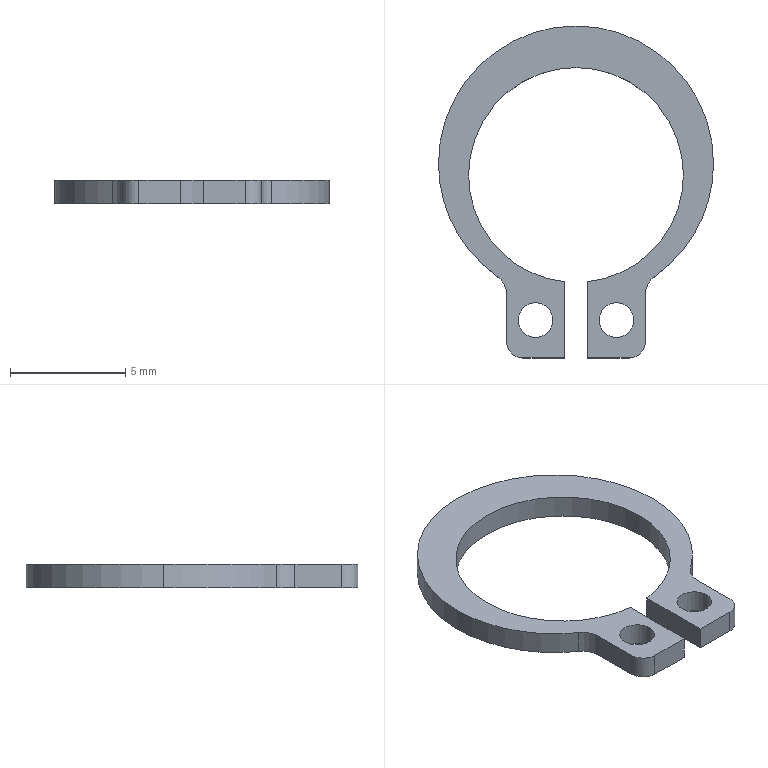Part | SolidWorks | features MoveCopyBody 1, Stock 1 | 1 solid | 22 faces | box 11.91 x 14.373 x 1 mm | volume 52.893 mm3 | cylinder 14 | plane 8 | commonest cylinder face diameters 1.5 x4 9.3 x3 11.91 x3 1.4 x2 2 x2
STEP:
#1=CARTESIAN_POINT('',(1.,-6.286,1.));
#2=VERTEX_POINT('',#1);
#3=CARTESIAN_POINT('',(2.5,-6.286,1.));
#4=VERTEX_POINT('',#3);
#5=CARTESIAN_POINT('',(1.75,-6.286,1.));
#6=DIRECTION('',(0.,0.,1.));
#7=DIRECTION('',(-1.,0.,0.));
#8=AXIS2_PLACEMENT_3D('',#5,#6,#7);
#9=CIRCLE('',#8,0.75);
#10=EDGE_CURVE('',#2,#4,#9,.T.);
#11=ORIENTED_EDGE('',*,*,#10,.T.);
#12=CARTESIAN_POINT('',(2.5,-6.286,0.));
#13=VERTEX_POINT('',#12);
#14=CARTESIAN_POINT('',(2.5,-6.286,1.));
#15=DIRECTION('',(0.,0.,-1.));
#16=VECTOR('',#15,1000.);
#17=LINE('',#14,#16);
#18=EDGE_CURVE('',#4,#13,#17,.T.);
#19=ORIENTED_EDGE('',*,*,#18,.T.);
#20=CARTESIAN_POINT('',(1.,-6.286,0.));
#21=VERTEX_POINT('',#20);
#22=CARTESIAN_POINT('',(1.75,-6.286,0.));
#23=DIRECTION('',(0.,0.,1.));
#24=DIRECTION('',(-1.,0.,0.));
#25=AXIS2_PLACEMENT_3D('',#22,#23,#24);
#26=CIRCLE('',#25,0.75);
#27=EDGE_CURVE('',#21,#13,#26,.T.);
#28=ORIENTED_EDGE('',*,*,#27,.F.);
#29=CARTESIAN_POINT('',(1.,-6.286,1.));
#30=DIRECTION('',(0.,0.,-1.));
#31=VECTOR('',#30,1000.);
#32=LINE('',#29,#31);
#33=EDGE_CURVE('',#2,#21,#32,.T.);
#34=ORIENTED_EDGE('',*,*,#33,.F.);
#35=EDGE_LOOP('',(#11,#19,#28,#34));
#36=FACE_OUTER_BOUND('',#35,.T.);
#37=CARTESIAN_POINT('',(1.75,-6.286,1.));
#38=DIRECTION('',(0.,0.,-1.));
#39=DIRECTION('',(-1.,0.,0.));
#40=AXIS2_PLACEMENT_3D('',#37,#38,#39);
#41=CYLINDRICAL_SURFACE('',#40,0.75);
#42=ADVANCED_FACE('',(#36),#41,.F.);
#43=CARTESIAN_POINT('',(-2.5,-6.286,1.));
#44=VERTEX_POINT('',#43);
#45=CARTESIAN_POINT('',(-1.,-6.286,1.));
#46=VERTEX_POINT('',#45);
#47=CARTESIAN_POINT('',(-1.75,-6.286,1.));
#48=DIRECTION('',(0.,0.,1.));
#49=DIRECTION('',(1.,0.,0.));
#50=AXIS2_PLACEMENT_3D('',#47,#48,#49);
#51=CIRCLE('',#50,0.75);
#52=EDGE_CURVE('',#44,#46,#51,.T.);
#53=ORIENTED_EDGE('',*,*,#52,.T.);
#54=CARTESIAN_POINT('',(-1.,-6.286,0.));
#55=VERTEX_POINT('',#54);
#56=CARTESIAN_POINT('',(-1.,-6.286,1.));
#57=DIRECTION('',(0.,0.,-1.));
#58=VECTOR('',#57,1000.);
#59=LINE('',#56,#58);
#60=EDGE_CURVE('',#46,#55,#59,.T.);
#61=ORIENTED_EDGE('',*,*,#60,.T.);
#62=CARTESIAN_POINT('',(-2.5,-6.286,0.));
#63=VERTEX_POINT('',#62);
#64=CARTESIAN_POINT('',(-1.75,-6.286,0.));
#65=DIRECTION('',(0.,0.,1.));
#66=DIRECTION('',(1.,0.,0.));
#67=AXIS2_PLACEMENT_3D('',#64,#65,#66);
#68=CIRCLE('',#67,0.75);
#69=EDGE_CURVE('',#63,#55,#68,.T.);
#70=ORIENTED_EDGE('',*,*,#69,.F.);
#71=CARTESIAN_POINT('',(-2.5,-6.286,1.));
#72=DIRECTION('',(0.,0.,-1.));
#73=VECTOR('',#72,1000.);
#74=LINE('',#71,#73);
#75=EDGE_CURVE('',#44,#63,#74,.T.);
#76=ORIENTED_EDGE('',*,*,#75,.F.);
#77=EDGE_LOOP('',(#53,#61,#70,#76));
#78=FACE_OUTER_BOUND('',#77,.T.);
#79=CARTESIAN_POINT('',(-1.75,-6.286,1.));
#80=DIRECTION('',(0.,0.,-1.));
#81=DIRECTION('',(-1.,0.,0.));
#82=AXIS2_PLACEMENT_3D('',#79,#80,#81);
#83=CYLINDRICAL_SURFACE('',#82,0.75);
#84=ADVANCED_FACE('',(#78),#83,.F.);
#85=CARTESIAN_POINT('',(5.955,0.495,1.));
#86=VERTEX_POINT('',#85);
#87=CARTESIAN_POINT('',(-5.955,0.495,1.));
#88=VERTEX_POINT('',#87);
#89=CARTESIAN_POINT('',(0.,0.495,1.));
#90=DIRECTION('',(0.,0.,1.));
#91=DIRECTION('',(1.,0.,0.));
#92=AXIS2_PLACEMENT_3D('',#89,#90,#91);
#93=CIRCLE('',#92,5.955);
#94=EDGE_CURVE('',#86,#88,#93,.T.);
#95=ORIENTED_EDGE('',*,*,#94,.F.);
#96=CARTESIAN_POINT('',(5.955,0.495,0.));
#97=VERTEX_POINT('',#96);
#98=CARTESIAN_POINT('',(5.955,0.495,1.));
#99=DIRECTION('',(0.,0.,-1.));
#100=VECTOR('',#99,1000.);
#101=LINE('',#98,#100);
#102=EDGE_CURVE('',#86,#97,#101,.T.);
#103=ORIENTED_EDGE('',*,*,#102,.T.);
#104=CARTESIAN_POINT('',(-5.955,0.495,0.));
#105=VERTEX_POINT('',#104);
#106=CARTESIAN_POINT('',(0.,0.495,0.));
#107=DIRECTION('',(0.,0.,1.));
#108=DIRECTION('',(1.,0.,0.));
#109=AXIS2_PLACEMENT_3D('',#106,#107,#108);
#110=CIRCLE('',#109,5.955);
#111=EDGE_CURVE('',#97,#105,#110,.T.);
#112=ORIENTED_EDGE('',*,*,#111,.T.);
#113=CARTESIAN_POINT('',(-5.955,0.495,1.));
#114=DIRECTION('',(0.,0.,-1.));
#115=VECTOR('',#114,1000.);
#116=LINE('',#113,#115);
#117=EDGE_CURVE('',#88,#105,#116,.T.);
#118=ORIENTED_EDGE('',*,*,#117,.F.);
#119=EDGE_LOOP('',(#95,#103,#112,#118));
#120=FACE_OUTER_BOUND('',#119,.T.);
#121=CARTESIAN_POINT('',(0.,0.495,1.));
#122=DIRECTION('',(0.,0.,-1.));
#123=DIRECTION('',(-1.,0.,0.));
#124=AXIS2_PLACEMENT_3D('',#121,#122,#123);
#125=CYLINDRICAL_SURFACE('',#124,5.955);
#126=ADVANCED_FACE('',(#120),#125,.T.);
#127=CARTESIAN_POINT('',(-3.425,-4.377,1.));
#128=VERTEX_POINT('',#127);
#129=CARTESIAN_POINT('',(0.,0.495,1.));
#130=DIRECTION('',(0.,0.,1.));
#131=DIRECTION('',(1.,0.,0.));
#132=AXIS2_PLACEMENT_3D('',#129,#130,#131);
#133=CIRCLE('',#132,5.955);
#134=EDGE_CURVE('',#88,#128,#133,.T.);
#135=ORIENTED_EDGE('',*,*,#134,.F.);
#136=ORIENTED_EDGE('',*,*,#117,.T.);
#137=CARTESIAN_POINT('',(-3.425,-4.377,0.));
#138=VERTEX_POINT('',#137);
#139=CARTESIAN_POINT('',(0.,0.495,0.));
#140=DIRECTION('',(0.,0.,1.));
#141=DIRECTION('',(1.,0.,0.));
#142=AXIS2_PLACEMENT_3D('',#139,#140,#141);
#143=CIRCLE('',#142,5.955);
#144=EDGE_CURVE('',#105,#138,#143,.T.);
#145=ORIENTED_EDGE('',*,*,#144,.T.);
#146=CARTESIAN_POINT('',(-3.425,-4.377,1.));
#147=DIRECTION('',(0.,0.,1.));
#148=VECTOR('',#147,1000.);
#149=LINE('',#146,#148);
#150=EDGE_CURVE('',#138,#128,#149,.T.);
#151=ORIENTED_EDGE('',*,*,#150,.T.);
#152=EDGE_LOOP('',(#135,#136,#145,#151));
#153=FACE_OUTER_BOUND('',#152,.T.);
#154=CARTESIAN_POINT('',(0.,0.495,1.));
#155=DIRECTION('',(0.,0.,-1.));
#156=DIRECTION('',(-1.,0.,0.));
#157=AXIS2_PLACEMENT_3D('',#154,#155,#156);
#158=CYLINDRICAL_SURFACE('',#157,5.955);
#159=ADVANCED_FACE('',(#153),#158,.T.);
#160=CARTESIAN_POINT('',(4.65,0.,1.));
#161=VERTEX_POINT('',#160);
#162=CARTESIAN_POINT('',(0.5,-4.623,1.));
#163=VERTEX_POINT('',#162);
#164=CARTESIAN_POINT('',(0.,0.,1.));
#165=DIRECTION('',(0.,0.,-1.));
#166=DIRECTION('',(1.,0.,0.));
#167=AXIS2_PLACEMENT_3D('',#164,#165,#166);
#168=CIRCLE('',#167,4.65);
#169=EDGE_CURVE('',#161,#163,#168,.T.);
#170=ORIENTED_EDGE('',*,*,#169,.F.);
#171=CARTESIAN_POINT('',(4.65,0.,0.));
#172=VERTEX_POINT('',#171);
#173=CARTESIAN_POINT('',(4.65,0.,1.));
#174=DIRECTION('',(0.,0.,-1.));
#175=VECTOR('',#174,1000.);
#176=LINE('',#173,#175);
#177=EDGE_CURVE('',#161,#172,#176,.T.);
#178=ORIENTED_EDGE('',*,*,#177,.T.);
#179=CARTESIAN_POINT('',(0.5,-4.623,0.));
#180=VERTEX_POINT('',#179);
#181=CARTESIAN_POINT('',(0.,0.,0.));
#182=DIRECTION('',(0.,0.,-1.));
#183=DIRECTION('',(1.,0.,0.));
#184=AXIS2_PLACEMENT_3D('',#181,#182,#183);
#185=CIRCLE('',#184,4.65);
#186=EDGE_CURVE('',#172,#180,#185,.T.);
#187=ORIENTED_EDGE('',*,*,#186,.T.);
#188=CARTESIAN_POINT('',(0.5,-4.623,1.));
#189=DIRECTION('',(0.,0.,-1.));
#190=VECTOR('',#189,1000.);
#191=LINE('',#188,#190);
#192=EDGE_CURVE('',#163,#180,#191,.T.);
#193=ORIENTED_EDGE('',*,*,#192,.F.);
#194=EDGE_LOOP('',(#170,#178,#187,#193));
#195=FACE_OUTER_BOUND('',#194,.T.);
#196=CARTESIAN_POINT('',(0.,0.,1.));
#197=DIRECTION('',(0.,0.,-1.));
#198=DIRECTION('',(-1.,0.,0.));
#199=AXIS2_PLACEMENT_3D('',#196,#197,#198);
#200=CYLINDRICAL_SURFACE('',#199,4.65);
#201=ADVANCED_FACE('',(#195),#200,.F.);
#202=ORIENTED_EDGE('',*,*,#177,.F.);
#203=CARTESIAN_POINT('',(-4.65,0.,1.));
#204=VERTEX_POINT('',#203);
#205=CARTESIAN_POINT('',(0.,0.,1.));
#206=DIRECTION('',(0.,0.,-1.));
#207=DIRECTION('',(1.,0.,0.));
#208=AXIS2_PLACEMENT_3D('',#205,#206,#207);
#209=CIRCLE('',#208,4.65);
#210=EDGE_CURVE('',#204,#161,#209,.T.);
#211=ORIENTED_EDGE('',*,*,#210,.F.);
#212=CARTESIAN_POINT('',(-4.65,0.,0.));
#213=VERTEX_POINT('',#212);
#214=CARTESIAN_POINT('',(-4.65,0.,1.));
#215=DIRECTION('',(0.,0.,-1.));
#216=VECTOR('',#215,1000.);
#217=LINE('',#214,#216);
#218=EDGE_CURVE('',#204,#213,#217,.T.);
#219=ORIENTED_EDGE('',*,*,#218,.T.);
#220=CARTESIAN_POINT('',(0.,0.,0.));
#221=DIRECTION('',(0.,0.,-1.));
#222=DIRECTION('',(1.,0.,0.));
#223=AXIS2_PLACEMENT_3D('',#220,#221,#222);
#224=CIRCLE('',#223,4.65);
#225=EDGE_CURVE('',#213,#172,#224,.T.);
#226=ORIENTED_EDGE('',*,*,#225,.T.);
#227=EDGE_LOOP('',(#202,#211,#219,#226));
#228=FACE_OUTER_BOUND('',#227,.T.);
#229=CARTESIAN_POINT('',(0.,0.,1.));
#230=DIRECTION('',(0.,0.,-1.));
#231=DIRECTION('',(-1.,0.,0.));
#232=AXIS2_PLACEMENT_3D('',#229,#230,#231);
#233=CYLINDRICAL_SURFACE('',#232,4.65);
#234=ADVANCED_FACE('',(#228),#233,.F.);
#235=ORIENTED_EDGE('',*,*,#52,.F.);
#236=CARTESIAN_POINT('',(-1.75,-6.286,1.));
#237=DIRECTION('',(0.,0.,1.));
#238=DIRECTION('',(1.,0.,0.));
#239=AXIS2_PLACEMENT_3D('',#236,#237,#238);
#240=CIRCLE('',#239,0.75);
#241=EDGE_CURVE('',#46,#44,#240,.T.);
#242=ORIENTED_EDGE('',*,*,#241,.F.);
#243=EDGE_LOOP('',(#235,#242));
#244=FACE_BOUND('',#243,.T.);
#245=CARTESIAN_POINT('',(0.5,-7.923,1.));
#246=VERTEX_POINT('',#245);
#247=CARTESIAN_POINT('',(2.3,-7.923,1.));
#248=VERTEX_POINT('',#247);
#249=CARTESIAN_POINT('',(0.5,-7.923,1.));
#250=DIRECTION('',(1.,0.,0.));
#251=VECTOR('',#250,1000.);
#252=LINE('',#249,#251);
#253=EDGE_CURVE('',#246,#248,#252,.T.);
#254=ORIENTED_EDGE('',*,*,#253,.T.);
#255=CARTESIAN_POINT('',(3.,-7.223,1.));
#256=VERTEX_POINT('',#255);
#257=CARTESIAN_POINT('',(2.3,-7.223,1.));
#258=DIRECTION('',(0.,0.,1.));
#259=DIRECTION('',(1.,0.,0.));
#260=AXIS2_PLACEMENT_3D('',#257,#258,#259);
#261=CIRCLE('',#260,0.7);
#262=EDGE_CURVE('',#248,#256,#261,.T.);
#263=ORIENTED_EDGE('',*,*,#262,.T.);
#264=CARTESIAN_POINT('',(3.,-5.195,1.));
#265=VERTEX_POINT('',#264);
#266=CARTESIAN_POINT('',(3.,-7.923,1.));
#267=DIRECTION('',(0.,1.,0.));
#268=VECTOR('',#267,1000.);
#269=LINE('',#266,#268);
#270=EDGE_CURVE('',#256,#265,#269,.T.);
#271=ORIENTED_EDGE('',*,*,#270,.T.);
#272=CARTESIAN_POINT('',(3.425,-4.377,1.));
#273=VERTEX_POINT('',#272);
#274=CARTESIAN_POINT('',(4.,-5.195,1.));
#275=DIRECTION('',(0.,0.,-1.));
#276=DIRECTION('',(1.,0.,0.));
#277=AXIS2_PLACEMENT_3D('',#274,#275,#276);
#278=CIRCLE('',#277,1.);
#279=EDGE_CURVE('',#265,#273,#278,.T.);
#280=ORIENTED_EDGE('',*,*,#279,.T.);
#281=CARTESIAN_POINT('',(0.,0.495,1.));
#282=DIRECTION('',(0.,0.,1.));
#283=DIRECTION('',(1.,0.,0.));
#284=AXIS2_PLACEMENT_3D('',#281,#282,#283);
#285=CIRCLE('',#284,5.955);
#286=EDGE_CURVE('',#273,#86,#285,.T.);
#287=ORIENTED_EDGE('',*,*,#286,.T.);
#288=ORIENTED_EDGE('',*,*,#94,.T.);
#289=ORIENTED_EDGE('',*,*,#134,.T.);
#290=CARTESIAN_POINT('',(-3.,-5.195,1.));
#291=VERTEX_POINT('',#290);
#292=CARTESIAN_POINT('',(-4.,-5.195,1.));
#293=DIRECTION('',(0.,0.,-1.));
#294=DIRECTION('',(1.,0.,0.));
#295=AXIS2_PLACEMENT_3D('',#292,#293,#294);
#296=CIRCLE('',#295,1.);
#297=EDGE_CURVE('',#128,#291,#296,.T.);
#298=ORIENTED_EDGE('',*,*,#297,.T.);
#299=CARTESIAN_POINT('',(-3.,-7.223,1.));
#300=VERTEX_POINT('',#299);
#301=CARTESIAN_POINT('',(-3.,-7.923,1.));
#302=DIRECTION('',(0.,-1.,0.));
#303=VECTOR('',#302,1000.);
#304=LINE('',#301,#303);
#305=EDGE_CURVE('',#291,#300,#304,.T.);
#306=ORIENTED_EDGE('',*,*,#305,.T.);
#307=CARTESIAN_POINT('',(-2.3,-7.923,1.));
#308=VERTEX_POINT('',#307);
#309=CARTESIAN_POINT('',(-2.3,-7.223,1.));
#310=DIRECTION('',(0.,0.,1.));
#311=DIRECTION('',(1.,0.,0.));
#312=AXIS2_PLACEMENT_3D('',#309,#310,#311);
#313=CIRCLE('',#312,0.7);
#314=EDGE_CURVE('',#300,#308,#313,.T.);
#315=ORIENTED_EDGE('',*,*,#314,.T.);
#316=CARTESIAN_POINT('',(-0.5,-7.923,1.));
#317=VERTEX_POINT('',#316);
#318=CARTESIAN_POINT('',(-0.5,-7.923,1.));
#319=DIRECTION('',(1.,0.,0.));
#320=VECTOR('',#319,1000.);
#321=LINE('',#318,#320);
#322=EDGE_CURVE('',#308,#317,#321,.T.);
#323=ORIENTED_EDGE('',*,*,#322,.T.);
#324=CARTESIAN_POINT('',(-0.5,-4.623,1.));
#325=VERTEX_POINT('',#324);
#326=CARTESIAN_POINT('',(-0.5,-4.623,1.));
#327=DIRECTION('',(0.,1.,0.));
#328=VECTOR('',#327,1000.);
#329=LINE('',#326,#328);
#330=EDGE_CURVE('',#317,#325,#329,.T.);
#331=ORIENTED_EDGE('',*,*,#330,.T.);
#332=CARTESIAN_POINT('',(0.,0.,1.));
#333=DIRECTION('',(0.,0.,-1.));
#334=DIRECTION('',(1.,0.,0.));
#335=AXIS2_PLACEMENT_3D('',#332,#333,#334);
#336=CIRCLE('',#335,4.65);
#337=EDGE_CURVE('',#325,#204,#336,.T.);
#338=ORIENTED_EDGE('',*,*,#337,.T.);
#339=ORIENTED_EDGE('',*,*,#210,.T.);
#340=ORIENTED_EDGE('',*,*,#169,.T.);
#341=CARTESIAN_POINT('',(0.5,-4.623,1.));
#342=DIRECTION('',(0.,-1.,0.));
#343=VECTOR('',#342,1000.);
#344=LINE('',#341,#343);
#345=EDGE_CURVE('',#163,#246,#344,.T.);
#346=ORIENTED_EDGE('',*,*,#345,.T.);
#347=EDGE_LOOP('',(#254,#263,#271,#280,#287,#288,#289,#298,#306,#315,#323,#331,#338,#339,#340,#346));
#348=FACE_OUTER_BOUND('',#347,.T.);
#349=ORIENTED_EDGE('',*,*,#10,.F.);
#350=CARTESIAN_POINT('',(1.75,-6.286,1.));
#351=DIRECTION('',(0.,0.,1.));
#352=DIRECTION('',(-1.,0.,0.));
#353=AXIS2_PLACEMENT_3D('',#350,#351,#352);
#354=CIRCLE('',#353,0.75);
#355=EDGE_CURVE('',#4,#2,#354,.T.);
#356=ORIENTED_EDGE('',*,*,#355,.F.);
#357=EDGE_LOOP('',(#349,#356));
#358=FACE_BOUND('',#357,.T.);
#359=CARTESIAN_POINT('',(0.,0.,1.));
#360=DIRECTION('',(0.,0.,1.));
#361=DIRECTION('',(1.,0.,0.));
#362=AXIS2_PLACEMENT_3D('',#359,#360,#361);
#363=PLANE('',#362);
#364=ADVANCED_FACE('',(#244,#348,#358),#363,.T.);
#365=ORIENTED_EDGE('',*,*,#69,.T.);
#366=CARTESIAN_POINT('',(-1.75,-6.286,0.));
#367=DIRECTION('',(0.,0.,1.));
#368=DIRECTION('',(1.,0.,0.));
#369=AXIS2_PLACEMENT_3D('',#366,#367,#368);
#370=CIRCLE('',#369,0.75);
#371=EDGE_CURVE('',#55,#63,#370,.T.);
#372=ORIENTED_EDGE('',*,*,#371,.T.);
#373=EDGE_LOOP('',(#365,#372));
#374=FACE_BOUND('',#373,.T.);
#375=CARTESIAN_POINT('',(3.,-7.223,0.));
#376=VERTEX_POINT('',#375);
#377=CARTESIAN_POINT('',(3.,-5.195,0.));
#378=VERTEX_POINT('',#377);
#379=CARTESIAN_POINT('',(3.,-7.923,0.));
#380=DIRECTION('',(0.,1.,0.));
#381=VECTOR('',#380,1000.);
#382=LINE('',#379,#381);
#383=EDGE_CURVE('',#376,#378,#382,.T.);
#384=ORIENTED_EDGE('',*,*,#383,.F.);
#385=CARTESIAN_POINT('',(2.3,-7.923,0.));
#386=VERTEX_POINT('',#385);
#387=CARTESIAN_POINT('',(2.3,-7.223,0.));
#388=DIRECTION('',(0.,0.,-1.));
#389=DIRECTION('',(1.,0.,0.));
#390=AXIS2_PLACEMENT_3D('',#387,#388,#389);
#391=CIRCLE('',#390,0.7);
#392=EDGE_CURVE('',#376,#386,#391,.T.);
#393=ORIENTED_EDGE('',*,*,#392,.T.);
#394=CARTESIAN_POINT('',(0.5,-7.923,0.));
#395=VERTEX_POINT('',#394);
#396=CARTESIAN_POINT('',(0.5,-7.923,0.));
#397=DIRECTION('',(1.,0.,0.));
#398=VECTOR('',#397,1000.);
#399=LINE('',#396,#398);
#400=EDGE_CURVE('',#395,#386,#399,.T.);
#401=ORIENTED_EDGE('',*,*,#400,.F.);
#402=CARTESIAN_POINT('',(0.5,-4.623,0.));
#403=DIRECTION('',(0.,-1.,0.));
#404=VECTOR('',#403,1000.);
#405=LINE('',#402,#404);
#406=EDGE_CURVE('',#180,#395,#405,.T.);
#407=ORIENTED_EDGE('',*,*,#406,.F.);
#408=ORIENTED_EDGE('',*,*,#186,.F.);
#409=ORIENTED_EDGE('',*,*,#225,.F.);
#410=CARTESIAN_POINT('',(-0.5,-4.623,0.));
#411=VERTEX_POINT('',#410);
#412=CARTESIAN_POINT('',(0.,0.,0.));
#413=DIRECTION('',(0.,0.,-1.));
#414=DIRECTION('',(1.,0.,0.));
#415=AXIS2_PLACEMENT_3D('',#412,#413,#414);
#416=CIRCLE('',#415,4.65);
#417=EDGE_CURVE('',#411,#213,#416,.T.);
#418=ORIENTED_EDGE('',*,*,#417,.F.);
#419=CARTESIAN_POINT('',(-0.5,-7.923,0.));
#420=VERTEX_POINT('',#419);
#421=CARTESIAN_POINT('',(-0.5,-4.623,0.));
#422=DIRECTION('',(0.,1.,0.));
#423=VECTOR('',#422,1000.);
#424=LINE('',#421,#423);
#425=EDGE_CURVE('',#420,#411,#424,.T.);
#426=ORIENTED_EDGE('',*,*,#425,.F.);
#427=CARTESIAN_POINT('',(-2.3,-7.923,0.));
#428=VERTEX_POINT('',#427);
#429=CARTESIAN_POINT('',(-0.5,-7.923,0.));
#430=DIRECTION('',(1.,0.,0.));
#431=VECTOR('',#430,1000.);
#432=LINE('',#429,#431);
#433=EDGE_CURVE('',#428,#420,#432,.T.);
#434=ORIENTED_EDGE('',*,*,#433,.F.);
#435=CARTESIAN_POINT('',(-3.,-7.223,0.));
#436=VERTEX_POINT('',#435);
#437=CARTESIAN_POINT('',(-2.3,-7.223,0.));
#438=DIRECTION('',(0.,0.,-1.));
#439=DIRECTION('',(1.,0.,0.));
#440=AXIS2_PLACEMENT_3D('',#437,#438,#439);
#441=CIRCLE('',#440,0.7);
#442=EDGE_CURVE('',#428,#436,#441,.T.);
#443=ORIENTED_EDGE('',*,*,#442,.T.);
#444=CARTESIAN_POINT('',(-3.,-5.195,0.));
#445=VERTEX_POINT('',#444);
#446=CARTESIAN_POINT('',(-3.,-7.923,0.));
#447=DIRECTION('',(0.,-1.,0.));
#448=VECTOR('',#447,1000.);
#449=LINE('',#446,#448);
#450=EDGE_CURVE('',#445,#436,#449,.T.);
#451=ORIENTED_EDGE('',*,*,#450,.F.);
#452=CARTESIAN_POINT('',(-4.,-5.195,0.));
#453=DIRECTION('',(0.,0.,1.));
#454=DIRECTION('',(1.,0.,0.));
#455=AXIS2_PLACEMENT_3D('',#452,#453,#454);
#456=CIRCLE('',#455,1.);
#457=EDGE_CURVE('',#445,#138,#456,.T.);
#458=ORIENTED_EDGE('',*,*,#457,.T.);
#459=ORIENTED_EDGE('',*,*,#144,.F.);
#460=ORIENTED_EDGE('',*,*,#111,.F.);
#461=CARTESIAN_POINT('',(3.425,-4.377,0.));
#462=VERTEX_POINT('',#461);
#463=CARTESIAN_POINT('',(0.,0.495,0.));
#464=DIRECTION('',(0.,0.,1.));
#465=DIRECTION('',(1.,0.,0.));
#466=AXIS2_PLACEMENT_3D('',#463,#464,#465);
#467=CIRCLE('',#466,5.955);
#468=EDGE_CURVE('',#462,#97,#467,.T.);
#469=ORIENTED_EDGE('',*,*,#468,.F.);
#470=CARTESIAN_POINT('',(4.,-5.195,0.));
#471=DIRECTION('',(0.,0.,1.));
#472=DIRECTION('',(1.,0.,0.));
#473=AXIS2_PLACEMENT_3D('',#470,#471,#472);
#474=CIRCLE('',#473,1.);
#475=EDGE_CURVE('',#462,#378,#474,.T.);
#476=ORIENTED_EDGE('',*,*,#475,.T.);
#477=EDGE_LOOP('',(#384,#393,#401,#407,#408,#409,#418,#426,#434,#443,#451,#458,#459,#460,#469,#476));
#478=FACE_OUTER_BOUND('',#477,.T.);
#479=ORIENTED_EDGE('',*,*,#27,.T.);
#480=CARTESIAN_POINT('',(1.75,-6.286,0.));
#481=DIRECTION('',(0.,0.,1.));
#482=DIRECTION('',(-1.,0.,0.));
#483=AXIS2_PLACEMENT_3D('',#480,#481,#482);
#484=CIRCLE('',#483,0.75);
#485=EDGE_CURVE('',#13,#21,#484,.T.);
#486=ORIENTED_EDGE('',*,*,#485,.T.);
#487=EDGE_LOOP('',(#479,#486));
#488=FACE_BOUND('',#487,.T.);
#489=CARTESIAN_POINT('',(0.,0.,0.));
#490=DIRECTION('',(0.,0.,1.));
#491=DIRECTION('',(1.,0.,0.));
#492=AXIS2_PLACEMENT_3D('',#489,#490,#491);
#493=PLANE('',#492);
#494=ADVANCED_FACE('',(#374,#478,#488),#493,.F.);
#495=ORIENTED_EDGE('',*,*,#218,.F.);
#496=ORIENTED_EDGE('',*,*,#337,.F.);
#497=CARTESIAN_POINT('',(-0.5,-4.623,1.));
#498=DIRECTION('',(0.,0.,-1.));
#499=VECTOR('',#498,1000.);
#500=LINE('',#497,#499);
#501=EDGE_CURVE('',#325,#411,#500,.T.);
#502=ORIENTED_EDGE('',*,*,#501,.T.);
#503=ORIENTED_EDGE('',*,*,#417,.T.);
#504=EDGE_LOOP('',(#495,#496,#502,#503));
#505=FACE_OUTER_BOUND('',#504,.T.);
#506=CARTESIAN_POINT('',(0.,0.,1.));
#507=DIRECTION('',(0.,0.,-1.));
#508=DIRECTION('',(-1.,0.,0.));
#509=AXIS2_PLACEMENT_3D('',#506,#507,#508);
#510=CYLINDRICAL_SURFACE('',#509,4.65);
#511=ADVANCED_FACE('',(#505),#510,.F.);
#512=ORIENTED_EDGE('',*,*,#406,.T.);
#513=CARTESIAN_POINT('',(0.5,-7.923,1.));
#514=DIRECTION('',(0.,0.,-1.));
#515=VECTOR('',#514,1000.);
#516=LINE('',#513,#515);
#517=EDGE_CURVE('',#246,#395,#516,.T.);
#518=ORIENTED_EDGE('',*,*,#517,.F.);
#519=ORIENTED_EDGE('',*,*,#345,.F.);
#520=ORIENTED_EDGE('',*,*,#192,.T.);
#521=EDGE_LOOP('',(#512,#518,#519,#520));
#522=FACE_OUTER_BOUND('',#521,.T.);
#523=CARTESIAN_POINT('',(0.5,-4.623,1.));
#524=DIRECTION('',(1.,0.,0.));
#525=DIRECTION('',(0.,1.,0.));
#526=AXIS2_PLACEMENT_3D('',#523,#524,#525);
#527=PLANE('',#526);
#528=ADVANCED_FACE('',(#522),#527,.F.);
#529=ORIENTED_EDGE('',*,*,#400,.T.);
#530=CARTESIAN_POINT('',(2.3,-7.923,1.));
#531=DIRECTION('',(0.,0.,1.));
#532=VECTOR('',#531,1000.);
#533=LINE('',#530,#532);
#534=EDGE_CURVE('',#386,#248,#533,.T.);
#535=ORIENTED_EDGE('',*,*,#534,.T.);
#536=ORIENTED_EDGE('',*,*,#253,.F.);
#537=ORIENTED_EDGE('',*,*,#517,.T.);
#538=EDGE_LOOP('',(#529,#535,#536,#537));
#539=FACE_OUTER_BOUND('',#538,.T.);
#540=CARTESIAN_POINT('',(0.5,-7.923,1.));
#541=DIRECTION('',(0.,1.,0.));
#542=DIRECTION('',(-1.,0.,0.));
#543=AXIS2_PLACEMENT_3D('',#540,#541,#542);
#544=PLANE('',#543);
#545=ADVANCED_FACE('',(#539),#544,.F.);
#546=ORIENTED_EDGE('',*,*,#270,.F.);
#547=CARTESIAN_POINT('',(3.,-7.223,1.));
#548=DIRECTION('',(0.,0.,-1.));
#549=VECTOR('',#548,1000.);
#550=LINE('',#547,#549);
#551=EDGE_CURVE('',#256,#376,#550,.T.);
#552=ORIENTED_EDGE('',*,*,#551,.T.);
#553=ORIENTED_EDGE('',*,*,#383,.T.);
#554=CARTESIAN_POINT('',(3.,-5.195,1.));
#555=DIRECTION('',(0.,0.,1.));
#556=VECTOR('',#555,1000.);
#557=LINE('',#554,#556);
#558=EDGE_CURVE('',#378,#265,#557,.T.);
#559=ORIENTED_EDGE('',*,*,#558,.T.);
#560=EDGE_LOOP('',(#546,#552,#553,#559));
#561=FACE_OUTER_BOUND('',#560,.T.);
#562=CARTESIAN_POINT('',(3.,-7.923,1.));
#563=DIRECTION('',(-1.,0.,0.));
#564=DIRECTION('',(0.,0.,1.));
#565=AXIS2_PLACEMENT_3D('',#562,#563,#564);
#566=PLANE('',#565);
#567=ADVANCED_FACE('',(#561),#566,.F.);
#568=ORIENTED_EDGE('',*,*,#102,.F.);
#569=ORIENTED_EDGE('',*,*,#286,.F.);
#570=CARTESIAN_POINT('',(3.425,-4.377,1.));
#571=DIRECTION('',(0.,0.,-1.));
#572=VECTOR('',#571,1000.);
#573=LINE('',#570,#572);
#574=EDGE_CURVE('',#273,#462,#573,.T.);
#575=ORIENTED_EDGE('',*,*,#574,.T.);
#576=ORIENTED_EDGE('',*,*,#468,.T.);
#577=EDGE_LOOP('',(#568,#569,#575,#576));
#578=FACE_OUTER_BOUND('',#577,.T.);
#579=CARTESIAN_POINT('',(0.,0.495,1.));
#580=DIRECTION('',(0.,0.,-1.));
#581=DIRECTION('',(-1.,0.,0.));
#582=AXIS2_PLACEMENT_3D('',#579,#580,#581);
#583=CYLINDRICAL_SURFACE('',#582,5.955);
#584=ADVANCED_FACE('',(#578),#583,.T.);
#585=ORIENTED_EDGE('',*,*,#450,.T.);
#586=CARTESIAN_POINT('',(-3.,-7.223,1.));
#587=DIRECTION('',(0.,0.,1.));
#588=VECTOR('',#587,1000.);
#589=LINE('',#586,#588);
#590=EDGE_CURVE('',#436,#300,#589,.T.);
#591=ORIENTED_EDGE('',*,*,#590,.T.);
#592=ORIENTED_EDGE('',*,*,#305,.F.);
#593=CARTESIAN_POINT('',(-3.,-5.195,0.));
#594=DIRECTION('',(0.,0.,-1.));
#595=VECTOR('',#594,1000.);
#596=LINE('',#593,#595);
#597=EDGE_CURVE('',#291,#445,#596,.T.);
#598=ORIENTED_EDGE('',*,*,#597,.T.);
#599=EDGE_LOOP('',(#585,#591,#592,#598));
#600=FACE_OUTER_BOUND('',#599,.T.);
#601=CARTESIAN_POINT('',(-3.,-7.923,1.));
#602=DIRECTION('',(1.,0.,0.));
#603=DIRECTION('',(0.,0.,-1.));
#604=AXIS2_PLACEMENT_3D('',#601,#602,#603);
#605=PLANE('',#604);
#606=ADVANCED_FACE('',(#600),#605,.F.);
#607=ORIENTED_EDGE('',*,*,#322,.F.);
#608=CARTESIAN_POINT('',(-2.3,-7.923,1.));
#609=DIRECTION('',(0.,0.,-1.));
#610=VECTOR('',#609,1000.);
#611=LINE('',#608,#610);
#612=EDGE_CURVE('',#308,#428,#611,.T.);
#613=ORIENTED_EDGE('',*,*,#612,.T.);
#614=ORIENTED_EDGE('',*,*,#433,.T.);
#615=CARTESIAN_POINT('',(-0.5,-7.923,1.));
#616=DIRECTION('',(0.,0.,-1.));
#617=VECTOR('',#616,1000.);
#618=LINE('',#615,#617);
#619=EDGE_CURVE('',#317,#420,#618,.T.);
#620=ORIENTED_EDGE('',*,*,#619,.F.);
#621=EDGE_LOOP('',(#607,#613,#614,#620));
#622=FACE_OUTER_BOUND('',#621,.T.);
#623=CARTESIAN_POINT('',(-0.5,-7.923,1.));
#624=DIRECTION('',(0.,1.,0.));
#625=DIRECTION('',(0.,0.,1.));
#626=AXIS2_PLACEMENT_3D('',#623,#624,#625);
#627=PLANE('',#626);
#628=ADVANCED_FACE('',(#622),#627,.F.);
#629=ORIENTED_EDGE('',*,*,#425,.T.);
#630=ORIENTED_EDGE('',*,*,#501,.F.);
#631=ORIENTED_EDGE('',*,*,#330,.F.);
#632=ORIENTED_EDGE('',*,*,#619,.T.);
#633=EDGE_LOOP('',(#629,#630,#631,#632));
#634=FACE_OUTER_BOUND('',#633,.T.);
#635=CARTESIAN_POINT('',(-0.5,-4.623,1.));
#636=DIRECTION('',(-1.,0.,0.));
#637=DIRECTION('',(0.,-1.,0.));
#638=AXIS2_PLACEMENT_3D('',#635,#636,#637);
#639=PLANE('',#638);
#640=ADVANCED_FACE('',(#634),#639,.F.);
#641=ORIENTED_EDGE('',*,*,#60,.F.);
#642=ORIENTED_EDGE('',*,*,#241,.T.);
#643=ORIENTED_EDGE('',*,*,#75,.T.);
#644=ORIENTED_EDGE('',*,*,#371,.F.);
#645=EDGE_LOOP('',(#641,#642,#643,#644));
#646=FACE_OUTER_BOUND('',#645,.T.);
#647=CARTESIAN_POINT('',(-1.75,-6.286,1.));
#648=DIRECTION('',(0.,0.,-1.));
#649=DIRECTION('',(-1.,0.,0.));
#650=AXIS2_PLACEMENT_3D('',#647,#648,#649);
#651=CYLINDRICAL_SURFACE('',#650,0.75);
#652=ADVANCED_FACE('',(#646),#651,.F.);
#653=ORIENTED_EDGE('',*,*,#18,.F.);
#654=ORIENTED_EDGE('',*,*,#355,.T.);
#655=ORIENTED_EDGE('',*,*,#33,.T.);
#656=ORIENTED_EDGE('',*,*,#485,.F.);
#657=EDGE_LOOP('',(#653,#654,#655,#656));
#658=FACE_OUTER_BOUND('',#657,.T.);
#659=CARTESIAN_POINT('',(1.75,-6.286,1.));
#660=DIRECTION('',(0.,0.,-1.));
#661=DIRECTION('',(-1.,0.,0.));
#662=AXIS2_PLACEMENT_3D('',#659,#660,#661);
#663=CYLINDRICAL_SURFACE('',#662,0.75);
#664=ADVANCED_FACE('',(#658),#663,.F.);
#665=ORIENTED_EDGE('',*,*,#279,.F.);
#666=ORIENTED_EDGE('',*,*,#558,.F.);
#667=ORIENTED_EDGE('',*,*,#475,.F.);
#668=ORIENTED_EDGE('',*,*,#574,.F.);
#669=EDGE_LOOP('',(#665,#666,#667,#668));
#670=FACE_OUTER_BOUND('',#669,.T.);
#671=CARTESIAN_POINT('',(4.,-5.195,1.));
#672=DIRECTION('',(0.,0.,-1.));
#673=DIRECTION('',(-1.,0.,0.));
#674=AXIS2_PLACEMENT_3D('',#671,#672,#673);
#675=CYLINDRICAL_SURFACE('',#674,1.);
#676=ADVANCED_FACE('',(#670),#675,.F.);
#677=ORIENTED_EDGE('',*,*,#297,.F.);
#678=ORIENTED_EDGE('',*,*,#150,.F.);
#679=ORIENTED_EDGE('',*,*,#457,.F.);
#680=ORIENTED_EDGE('',*,*,#597,.F.);
#681=EDGE_LOOP('',(#677,#678,#679,#680));
#682=FACE_OUTER_BOUND('',#681,.T.);
#683=CARTESIAN_POINT('',(-4.,-5.195,1.));
#684=DIRECTION('',(0.,0.,-1.));
#685=DIRECTION('',(-1.,0.,0.));
#686=AXIS2_PLACEMENT_3D('',#683,#684,#685);
#687=CYLINDRICAL_SURFACE('',#686,1.);
#688=ADVANCED_FACE('',(#682),#687,.F.);
#689=ORIENTED_EDGE('',*,*,#262,.F.);
#690=ORIENTED_EDGE('',*,*,#534,.F.);
#691=ORIENTED_EDGE('',*,*,#392,.F.);
#692=ORIENTED_EDGE('',*,*,#551,.F.);
#693=EDGE_LOOP('',(#689,#690,#691,#692));
#694=FACE_OUTER_BOUND('',#693,.T.);
#695=CARTESIAN_POINT('',(2.3,-7.223,1.));
#696=DIRECTION('',(0.,0.,-1.));
#697=DIRECTION('',(-1.,0.,0.));
#698=AXIS2_PLACEMENT_3D('',#695,#696,#697);
#699=CYLINDRICAL_SURFACE('',#698,0.7);
#700=ADVANCED_FACE('',(#694),#699,.T.);
#701=ORIENTED_EDGE('',*,*,#314,.F.);
#702=ORIENTED_EDGE('',*,*,#590,.F.);
#703=ORIENTED_EDGE('',*,*,#442,.F.);
#704=ORIENTED_EDGE('',*,*,#612,.F.);
#705=EDGE_LOOP('',(#701,#702,#703,#704));
#706=FACE_OUTER_BOUND('',#705,.T.);
#707=CARTESIAN_POINT('',(-2.3,-7.223,1.));
#708=DIRECTION('',(0.,0.,-1.));
#709=DIRECTION('',(-1.,0.,0.));
#710=AXIS2_PLACEMENT_3D('',#707,#708,#709);
#711=CYLINDRICAL_SURFACE('',#710,0.7);
#712=ADVANCED_FACE('',(#706),#711,.T.);
#713=CLOSED_SHELL('',(#42,#84,#126,#159,#201,#234,#364,#494,#511,#528,#545,#567,#584,#606,#628,#640,#652,#664,#676,#688,#700,#712));
#714=MANIFOLD_SOLID_BREP('',#713);
#715=CARTESIAN_POINT('',(0.,0.,0.));
#716=DIRECTION('',(0.,0.,1.));
#717=DIRECTION('',(1.,0.,0.));
#718=AXIS2_PLACEMENT_3D('',#715,#716,#717);
#719=(LENGTH_UNIT()NAMED_UNIT(*)SI_UNIT(.MILLI.,.METRE.));
#720=UNCERTAINTY_MEASURE_WITH_UNIT(LENGTH_MEASURE(0.00001),#719,'','');
#721=(NAMED_UNIT(*)PLANE_ANGLE_UNIT()SI_UNIT($,.RADIAN.));
#722=(NAMED_UNIT(*)SI_UNIT($,.STERADIAN.)SOLID_ANGLE_UNIT());
#723=(GEOMETRIC_REPRESENTATION_CONTEXT(3)GLOBAL_UNCERTAINTY_ASSIGNED_CONTEXT((#720))GLOBAL_UNIT_ASSIGNED_CONTEXT((#719,#721,#722))REPRESENTATION_CONTEXT('',''));
#724=ADVANCED_BREP_SHAPE_REPRESENTATION('',(#714,#718),#723);